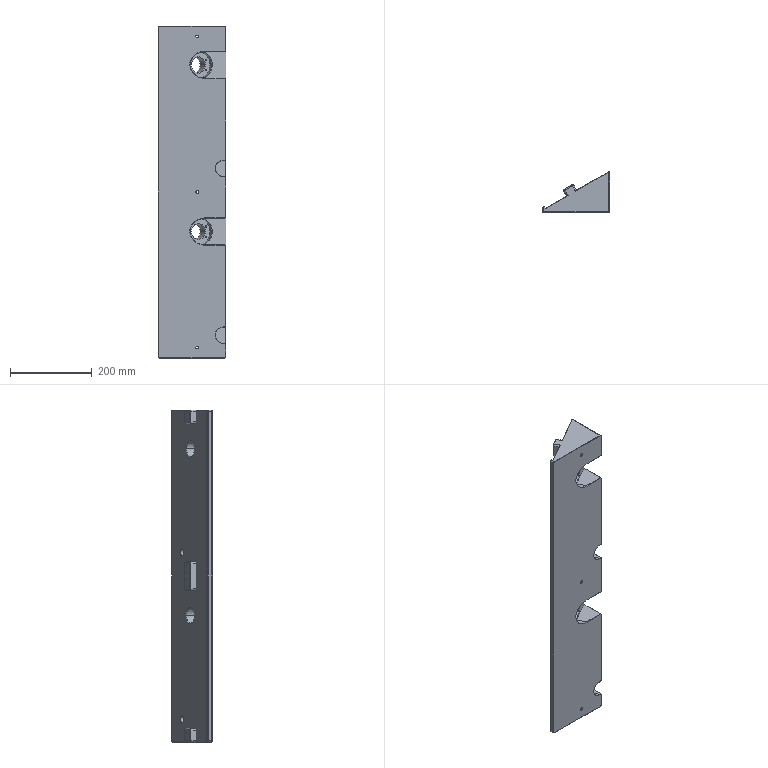Part | SolidWorks | features Chamfer 11, ICE 11, 3DProfileFeature 4, HoleWzd 4, Fillet 2, LPattern 2, CirPattern 1, Extrusion 1 | 1 solid | 245 faces | box 165 x 98.335 x 810.75 mm | volume 6353061 mm3 | plane 91 | cylinder 80 | cone 66 | spline 8 | commonest cylinder face diameters 3.3 x32 8 x16 7 x10 12 x6 16 x4 38 x4